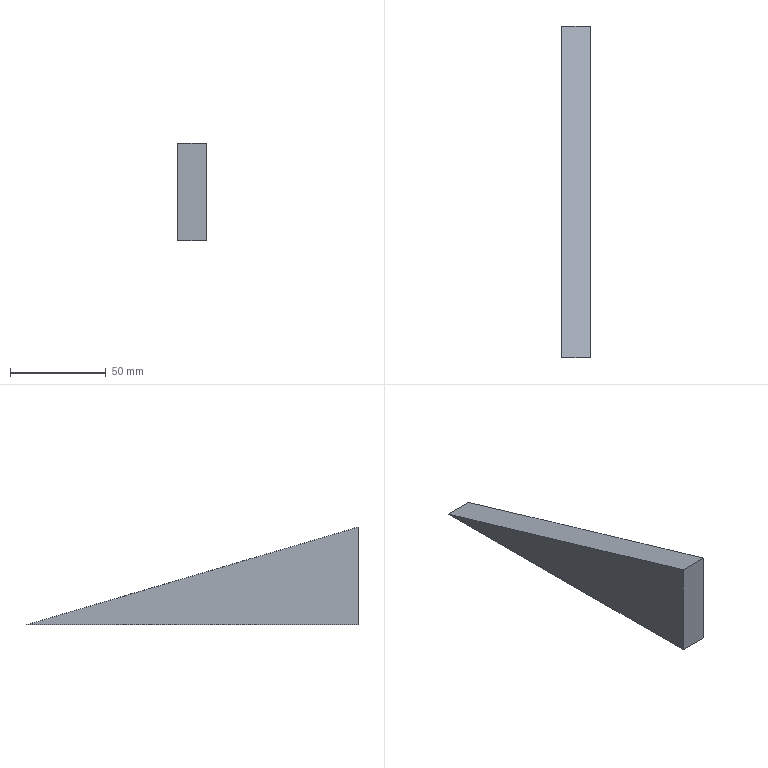Part | STEP file | 1 solid | 5 faces | box 15 x 173 x 50.952 mm | volume 66110 mm3 | plane 5
STEP:
#1=CARTESIAN_POINT('',(0.,0.,0.));
#2=DIRECTION('',(0.,0.,1.));
#3=DIRECTION('',(1.,0.,0.));
#4=AXIS2_PLACEMENT_3D('',#1,#2,#3);
#5=CARTESIAN_POINT('',(270.205,354.014,247.067));
#6=VERTEX_POINT('',#5);
#7=CARTESIAN_POINT('',(270.205,354.014,196.115));
#8=VERTEX_POINT('',#7);
#9=CARTESIAN_POINT('',(270.205,354.014,0.));
#10=DIRECTION('',(0.,0.,-1.));
#11=VECTOR('',#10,1.);
#12=LINE('',#9,#11);
#13=CARTESIAN_POINT('',(285.205,354.014,0.));
#14=DIRECTION('',(0.,1.,0.));
#15=DIRECTION('',(0.,0.,1.));
#16=AXIS2_PLACEMENT_3D('',#13,#14,#15);
#17=PLANE('',#16);
#18=CARTESIAN_POINT('',(0.,-15.));
#19=DIRECTION('',(-1.,0.));
#20=VECTOR('',#19,1.);
#21=LINE('',#18,#20);
#22=(GEOMETRIC_REPRESENTATION_CONTEXT(2)PARAMETRIC_REPRESENTATION_CONTEXT()REPRESENTATION_CONTEXT('',''));
#23=DEFINITIONAL_REPRESENTATION('',(#21),#22);
#24=PCURVE('',#17,#23);
#25=CARTESIAN_POINT('',(270.205,0.,0.));
#26=DIRECTION('',(-1.,0.,0.));
#27=DIRECTION('',(0.,0.,1.));
#28=AXIS2_PLACEMENT_3D('',#25,#26,#27);
#29=PLANE('',#28);
#30=CARTESIAN_POINT('',(0.,354.014));
#31=DIRECTION('',(-1.,0.));
#32=VECTOR('',#31,1.);
#33=LINE('',#30,#32);
#34=(GEOMETRIC_REPRESENTATION_CONTEXT(2)PARAMETRIC_REPRESENTATION_CONTEXT()REPRESENTATION_CONTEXT('',''));
#35=DEFINITIONAL_REPRESENTATION('',(#33),#34);
#36=PCURVE('',#29,#35);
#37=SURFACE_CURVE('',#12,(#24,#36),.PCURVE_S1.);
#38=EDGE_CURVE('',#6,#8,#37,.T.);
#39=ORIENTED_EDGE('',*,*,#38,.T.);
#40=CARTESIAN_POINT('',(285.205,354.014,196.115));
#41=VERTEX_POINT('',#40);
#42=CARTESIAN_POINT('',(285.205,354.014,196.115));
#43=DIRECTION('',(-1.,0.,0.));
#44=VECTOR('',#43,1.);
#45=LINE('',#42,#44);
#46=CARTESIAN_POINT('',(196.115,0.));
#47=DIRECTION('',(0.,-1.));
#48=VECTOR('',#47,1.);
#49=LINE('',#46,#48);
#50=(GEOMETRIC_REPRESENTATION_CONTEXT(2)PARAMETRIC_REPRESENTATION_CONTEXT()REPRESENTATION_CONTEXT('',''));
#51=DEFINITIONAL_REPRESENTATION('',(#49),#50);
#52=PCURVE('',#17,#51);
#53=CARTESIAN_POINT('',(285.205,0.,196.115));
#54=DIRECTION('',(0.,0.,1.));
#55=DIRECTION('',(1.,0.,0.));
#56=AXIS2_PLACEMENT_3D('',#53,#54,#55);
#57=PLANE('',#56);
#58=CARTESIAN_POINT('',(0.,354.014));
#59=DIRECTION('',(-1.,0.));
#60=VECTOR('',#59,1.);
#61=LINE('',#58,#60);
#62=(GEOMETRIC_REPRESENTATION_CONTEXT(2)PARAMETRIC_REPRESENTATION_CONTEXT()REPRESENTATION_CONTEXT('',''));
#63=DEFINITIONAL_REPRESENTATION('',(#61),#62);
#64=PCURVE('',#57,#63);
#65=SURFACE_CURVE('',#45,(#52,#64),.PCURVE_S1.);
#66=EDGE_CURVE('',#41,#8,#65,.T.);
#67=ORIENTED_EDGE('',*,*,#66,.F.);
#68=CARTESIAN_POINT('',(285.205,354.014,247.067));
#69=VERTEX_POINT('',#68);
#70=CARTESIAN_POINT('',(285.205,354.014,0.));
#71=DIRECTION('',(0.,0.,-1.));
#72=VECTOR('',#71,1.);
#73=LINE('',#70,#72);
#74=CARTESIAN_POINT('',(0.,0.));
#75=DIRECTION('',(-1.,0.));
#76=VECTOR('',#75,1.);
#77=LINE('',#74,#76);
#78=(GEOMETRIC_REPRESENTATION_CONTEXT(2)PARAMETRIC_REPRESENTATION_CONTEXT()REPRESENTATION_CONTEXT('',''));
#79=DEFINITIONAL_REPRESENTATION('',(#77),#78);
#80=PCURVE('',#17,#79);
#81=CARTESIAN_POINT('',(285.205,0.,0.));
#82=DIRECTION('',(-1.,0.,0.));
#83=DIRECTION('',(0.,0.,1.));
#84=AXIS2_PLACEMENT_3D('',#81,#82,#83);
#85=PLANE('',#84);
#86=CARTESIAN_POINT('',(0.,354.014));
#87=DIRECTION('',(-1.,0.));
#88=VECTOR('',#87,1.);
#89=LINE('',#86,#88);
#90=(GEOMETRIC_REPRESENTATION_CONTEXT(2)PARAMETRIC_REPRESENTATION_CONTEXT()REPRESENTATION_CONTEXT('',''));
#91=DEFINITIONAL_REPRESENTATION('',(#89),#90);
#92=PCURVE('',#85,#91);
#93=SURFACE_CURVE('',#73,(#80,#92),.PCURVE_S1.);
#94=EDGE_CURVE('',#69,#41,#93,.T.);
#95=ORIENTED_EDGE('',*,*,#94,.F.);
#96=CARTESIAN_POINT('',(285.205,354.014,247.067));
#97=DIRECTION('',(-1.,0.,0.));
#98=VECTOR('',#97,1.);
#99=LINE('',#96,#98);
#100=CARTESIAN_POINT('',(247.067,0.));
#101=DIRECTION('',(0.,-1.));
#102=VECTOR('',#101,1.);
#103=LINE('',#100,#102);
#104=(GEOMETRIC_REPRESENTATION_CONTEXT(2)PARAMETRIC_REPRESENTATION_CONTEXT()REPRESENTATION_CONTEXT('',''));
#105=DEFINITIONAL_REPRESENTATION('',(#103),#104);
#106=PCURVE('',#17,#105);
#107=CARTESIAN_POINT('',(285.205,95.215,323.288));
#108=DIRECTION('',(0.,-0.2825,-0.9593));
#109=DIRECTION('',(0.,0.9593,-0.2825));
#110=AXIS2_PLACEMENT_3D('',#107,#108,#109);
#111=PLANE('',#110);
#112=CARTESIAN_POINT('',(269.79,0.));
#113=DIRECTION('',(0.,-1.));
#114=VECTOR('',#113,1.);
#115=LINE('',#112,#114);
#116=(GEOMETRIC_REPRESENTATION_CONTEXT(2)PARAMETRIC_REPRESENTATION_CONTEXT()REPRESENTATION_CONTEXT('',''));
#117=DEFINITIONAL_REPRESENTATION('',(#115),#116);
#118=PCURVE('',#111,#117);
#119=SURFACE_CURVE('',#99,(#106,#118),.PCURVE_S1.);
#120=EDGE_CURVE('',#69,#6,#119,.T.);
#121=ORIENTED_EDGE('',*,*,#120,.T.);
#122=EDGE_LOOP('',(#39,#67,#95,#121));
#123=FACE_BOUND('',#122,.T.);
#124=ADVANCED_FACE('',(#123),#17,.F.);
#125=CARTESIAN_POINT('',(270.205,527.014,196.115));
#126=VERTEX_POINT('',#125);
#127=CARTESIAN_POINT('',(270.205,0.,196.115));
#128=DIRECTION('',(0.,1.,0.));
#129=VECTOR('',#128,1.);
#130=LINE('',#127,#129);
#131=CARTESIAN_POINT('',(-15.,0.));
#132=DIRECTION('',(0.,1.));
#133=VECTOR('',#132,1.);
#134=LINE('',#131,#133);
#135=(GEOMETRIC_REPRESENTATION_CONTEXT(2)PARAMETRIC_REPRESENTATION_CONTEXT()REPRESENTATION_CONTEXT('',''));
#136=DEFINITIONAL_REPRESENTATION('',(#134),#135);
#137=PCURVE('',#57,#136);
#138=CARTESIAN_POINT('',(196.115,0.));
#139=DIRECTION('',(0.,1.));
#140=VECTOR('',#139,1.);
#141=LINE('',#138,#140);
#142=(GEOMETRIC_REPRESENTATION_CONTEXT(2)PARAMETRIC_REPRESENTATION_CONTEXT()REPRESENTATION_CONTEXT('',''));
#143=DEFINITIONAL_REPRESENTATION('',(#141),#142);
#144=PCURVE('',#29,#143);
#145=SURFACE_CURVE('',#130,(#137,#144),.PCURVE_S1.);
#146=EDGE_CURVE('',#8,#126,#145,.T.);
#147=ORIENTED_EDGE('',*,*,#146,.T.);
#148=CARTESIAN_POINT('',(285.205,527.014,196.115));
#149=VERTEX_POINT('',#148);
#150=CARTESIAN_POINT('',(285.205,527.014,196.115));
#151=DIRECTION('',(-1.,0.,0.));
#152=VECTOR('',#151,1.);
#153=LINE('',#150,#152);
#154=CARTESIAN_POINT('',(0.,527.014));
#155=DIRECTION('',(-1.,0.));
#156=VECTOR('',#155,1.);
#157=LINE('',#154,#156);
#158=(GEOMETRIC_REPRESENTATION_CONTEXT(2)PARAMETRIC_REPRESENTATION_CONTEXT()REPRESENTATION_CONTEXT('',''));
#159=DEFINITIONAL_REPRESENTATION('',(#157),#158);
#160=PCURVE('',#57,#159);
#161=CARTESIAN_POINT('',(450.137,0.));
#162=DIRECTION('',(0.,-1.));
#163=VECTOR('',#162,1.);
#164=LINE('',#161,#163);
#165=(GEOMETRIC_REPRESENTATION_CONTEXT(2)PARAMETRIC_REPRESENTATION_CONTEXT()REPRESENTATION_CONTEXT('',''));
#166=DEFINITIONAL_REPRESENTATION('',(#164),#165);
#167=PCURVE('',#111,#166);
#168=SURFACE_CURVE('',#153,(#160,#167),.PCURVE_S1.);
#169=EDGE_CURVE('',#149,#126,#168,.T.);
#170=ORIENTED_EDGE('',*,*,#169,.F.);
#171=CARTESIAN_POINT('',(285.205,0.,196.115));
#172=DIRECTION('',(0.,1.,0.));
#173=VECTOR('',#172,1.);
#174=LINE('',#171,#173);
#175=CARTESIAN_POINT('',(0.,0.));
#176=DIRECTION('',(0.,1.));
#177=VECTOR('',#176,1.);
#178=LINE('',#175,#177);
#179=(GEOMETRIC_REPRESENTATION_CONTEXT(2)PARAMETRIC_REPRESENTATION_CONTEXT()REPRESENTATION_CONTEXT('',''));
#180=DEFINITIONAL_REPRESENTATION('',(#178),#179);
#181=PCURVE('',#57,#180);
#182=CARTESIAN_POINT('',(196.115,0.));
#183=DIRECTION('',(0.,1.));
#184=VECTOR('',#183,1.);
#185=LINE('',#182,#184);
#186=(GEOMETRIC_REPRESENTATION_CONTEXT(2)PARAMETRIC_REPRESENTATION_CONTEXT()REPRESENTATION_CONTEXT('',''));
#187=DEFINITIONAL_REPRESENTATION('',(#185),#186);
#188=PCURVE('',#85,#187);
#189=SURFACE_CURVE('',#174,(#181,#188),.PCURVE_S1.);
#190=EDGE_CURVE('',#41,#149,#189,.T.);
#191=ORIENTED_EDGE('',*,*,#190,.F.);
#192=ORIENTED_EDGE('',*,*,#66,.T.);
#193=EDGE_LOOP('',(#147,#170,#191,#192));
#194=FACE_BOUND('',#193,.T.);
#195=ADVANCED_FACE('',(#194),#57,.F.);
#196=CARTESIAN_POINT('',(270.205,95.215,323.288));
#197=DIRECTION('',(0.,-0.9593,0.2825));
#198=VECTOR('',#197,1.);
#199=LINE('',#196,#198);
#200=CARTESIAN_POINT('',(0.,-15.));
#201=DIRECTION('',(-1.,0.));
#202=VECTOR('',#201,1.);
#203=LINE('',#200,#202);
#204=(GEOMETRIC_REPRESENTATION_CONTEXT(2)PARAMETRIC_REPRESENTATION_CONTEXT()REPRESENTATION_CONTEXT('',''));
#205=DEFINITIONAL_REPRESENTATION('',(#203),#204);
#206=PCURVE('',#111,#205);
#207=CARTESIAN_POINT('',(323.288,95.215));
#208=DIRECTION('',(0.2825,-0.9593));
#209=VECTOR('',#208,1.);
#210=LINE('',#207,#209);
#211=(GEOMETRIC_REPRESENTATION_CONTEXT(2)PARAMETRIC_REPRESENTATION_CONTEXT()REPRESENTATION_CONTEXT('',''));
#212=DEFINITIONAL_REPRESENTATION('',(#210),#211);
#213=PCURVE('',#29,#212);
#214=SURFACE_CURVE('',#199,(#206,#213),.PCURVE_S1.);
#215=EDGE_CURVE('',#126,#6,#214,.T.);
#216=ORIENTED_EDGE('',*,*,#215,.T.);
#217=ORIENTED_EDGE('',*,*,#120,.F.);
#218=CARTESIAN_POINT('',(285.205,95.215,323.288));
#219=DIRECTION('',(0.,-0.9593,0.2825));
#220=VECTOR('',#219,1.);
#221=LINE('',#218,#220);
#222=CARTESIAN_POINT('',(0.,0.));
#223=DIRECTION('',(-1.,0.));
#224=VECTOR('',#223,1.);
#225=LINE('',#222,#224);
#226=(GEOMETRIC_REPRESENTATION_CONTEXT(2)PARAMETRIC_REPRESENTATION_CONTEXT()REPRESENTATION_CONTEXT('',''));
#227=DEFINITIONAL_REPRESENTATION('',(#225),#226);
#228=PCURVE('',#111,#227);
#229=CARTESIAN_POINT('',(323.288,95.215));
#230=DIRECTION('',(0.2825,-0.9593));
#231=VECTOR('',#230,1.);
#232=LINE('',#229,#231);
#233=(GEOMETRIC_REPRESENTATION_CONTEXT(2)PARAMETRIC_REPRESENTATION_CONTEXT()REPRESENTATION_CONTEXT('',''));
#234=DEFINITIONAL_REPRESENTATION('',(#232),#233);
#235=PCURVE('',#85,#234);
#236=SURFACE_CURVE('',#221,(#228,#235),.PCURVE_S1.);
#237=EDGE_CURVE('',#149,#69,#236,.T.);
#238=ORIENTED_EDGE('',*,*,#237,.F.);
#239=ORIENTED_EDGE('',*,*,#169,.T.);
#240=EDGE_LOOP('',(#216,#217,#238,#239));
#241=FACE_BOUND('',#240,.T.);
#242=ADVANCED_FACE('',(#241),#111,.F.);
#243=ORIENTED_EDGE('',*,*,#94,.T.);
#244=ORIENTED_EDGE('',*,*,#190,.T.);
#245=ORIENTED_EDGE('',*,*,#237,.T.);
#246=EDGE_LOOP('',(#243,#244,#245));
#247=FACE_BOUND('',#246,.T.);
#248=ADVANCED_FACE('',(#247),#85,.F.);
#249=ORIENTED_EDGE('',*,*,#38,.F.);
#250=ORIENTED_EDGE('',*,*,#215,.F.);
#251=ORIENTED_EDGE('',*,*,#146,.F.);
#252=EDGE_LOOP('',(#249,#250,#251));
#253=FACE_BOUND('',#252,.T.);
#254=ADVANCED_FACE('',(#253),#29,.T.);
#255=CLOSED_SHELL('',(#124,#195,#242,#248,#254));
#256=MANIFOLD_SOLID_BREP('',#255);
#257=(LENGTH_UNIT()NAMED_UNIT(*)SI_UNIT(.MILLI.,.METRE.));
#258=UNCERTAINTY_MEASURE_WITH_UNIT(LENGTH_MEASURE(0.0000001),#257,'','');
#259=(NAMED_UNIT(*)PLANE_ANGLE_UNIT()SI_UNIT($,.RADIAN.));
#260=(NAMED_UNIT(*)SI_UNIT($,.STERADIAN.)SOLID_ANGLE_UNIT());
#261=(GEOMETRIC_REPRESENTATION_CONTEXT(3)GLOBAL_UNCERTAINTY_ASSIGNED_CONTEXT((#258))GLOBAL_UNIT_ASSIGNED_CONTEXT((#257,#259,#260))REPRESENTATION_CONTEXT('',''));
#262=ADVANCED_BREP_SHAPE_REPRESENTATION('',(#4,#256),#261);